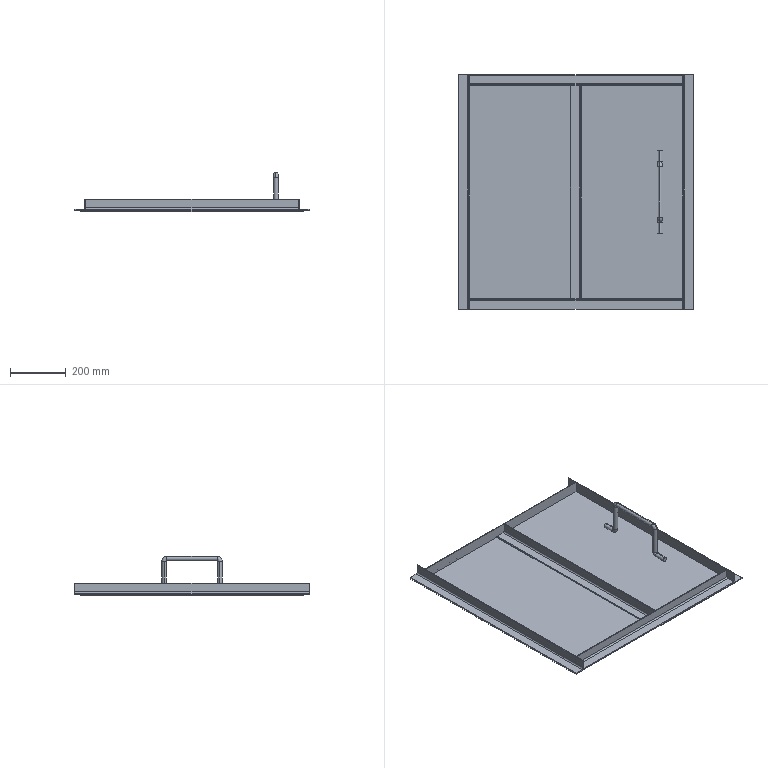Part | STEP file | Manhole door_Default<As machined> | 15 solids | 97 faces | box 840 x 840 x 140 mm | volume 3861650 mm3 | plane 64 | cylinder 25 | torus 8 | commonest cylinder face diameters 2.667 x10 16 x10 10 x5